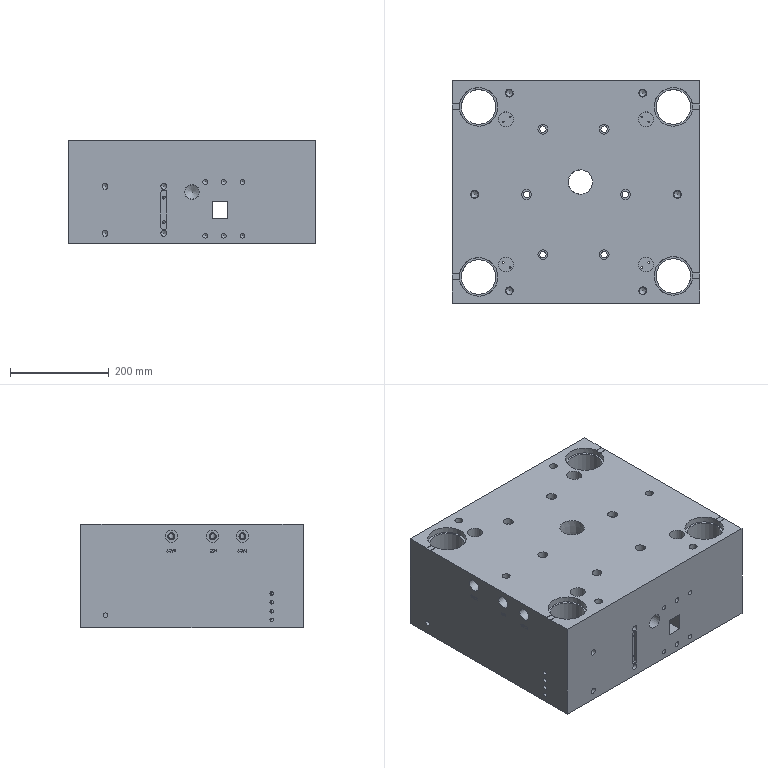Part | STEP file | AA | 1 solid | 800 faces | box 500 x 450 x 210 mm | volume 28750729 mm3 | plane 437 | cylinder 220 | cone 83 | other 50 | spline 6 | torus 4 | commonest cylinder face diameters 10 x57 20 x22 12 x15 8.5 x12 6 x10 8 x10